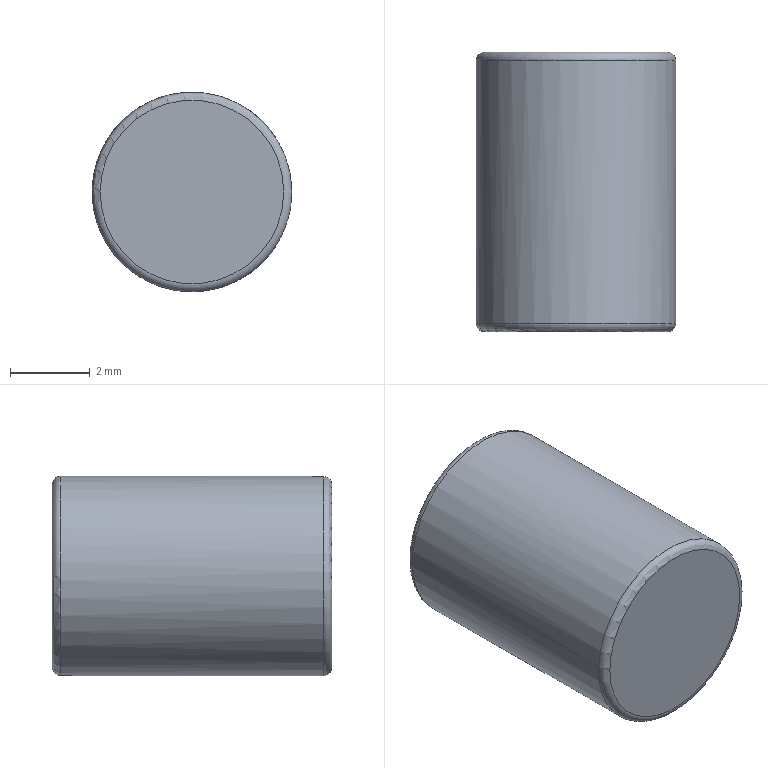Part | STEP file | Part [5] | 1 solid | 5 faces | box 5 x 7 x 5 mm | volume 137.18 mm3 | plane 2 | torus 2 | cylinder 1 | commonest cylinder face diameters 5 x1
STEP:
#1=CARTESIAN_POINT('',(-7.7,-134.3,0.));
#2=VERTEX_POINT('',#1);
#3=CARTESIAN_POINT('',(-10.,-134.3,0.));
#4=DIRECTION('',(0.,-1.,0.));
#5=DIRECTION('',(-1.,0.,0.));
#6=AXIS2_PLACEMENT_3D('',#3,#4,#5);
#7=CIRCLE('',#6,2.3);
#8=EDGE_CURVE('',#2,#2,#7,.T.);
#9=ORIENTED_EDGE('',*,*,#8,.T.);
#10=EDGE_LOOP('',(#9));
#11=FACE_BOUND('',#10,.T.);
#12=CARTESIAN_POINT('',(-10.,-134.3,0.));
#13=DIRECTION('',(0.,-1.,0.));
#14=DIRECTION('',(0.,0.,-1.));
#15=AXIS2_PLACEMENT_3D('',#12,#13,#14);
#16=PLANE('',#15);
#17=ADVANCED_FACE('',(#11),#16,.T.);
#18=CARTESIAN_POINT('',(-7.5,-134.1,0.));
#19=VERTEX_POINT('',#18);
#20=CARTESIAN_POINT('',(-7.5,-134.1,0.));
#21=CARTESIAN_POINT('',(-7.5,-134.1,0.05237));
#22=CARTESIAN_POINT('',(-7.503,-134.1,0.1571));
#23=CARTESIAN_POINT('',(-7.518,-134.1,0.3136));
#24=CARTESIAN_POINT('',(-7.543,-134.1,0.4688));
#25=CARTESIAN_POINT('',(-7.577,-134.1,0.6222));
#26=CARTESIAN_POINT('',(-7.621,-134.1,0.7732));
#27=CARTESIAN_POINT('',(-7.674,-134.1,0.9211));
#28=CARTESIAN_POINT('',(-7.737,-134.1,1.065));
#29=CARTESIAN_POINT('',(-7.808,-134.1,1.205));
#30=CARTESIAN_POINT('',(-7.888,-134.1,1.341));
#31=CARTESIAN_POINT('',(-7.976,-134.1,1.471));
#32=CARTESIAN_POINT('',(-8.073,-134.1,1.595));
#33=CARTESIAN_POINT('',(-8.177,-134.1,1.713));
#34=CARTESIAN_POINT('',(-8.288,-134.1,1.824));
#35=CARTESIAN_POINT('',(-8.406,-134.1,1.928));
#36=CARTESIAN_POINT('',(-8.53,-134.1,2.024));
#37=CARTESIAN_POINT('',(-8.66,-134.1,2.112));
#38=CARTESIAN_POINT('',(-8.795,-134.1,2.192));
#39=CARTESIAN_POINT('',(-8.935,-134.1,2.264));
#40=CARTESIAN_POINT('',(-9.08,-134.1,2.326));
#41=CARTESIAN_POINT('',(-9.227,-134.1,2.379));
#42=CARTESIAN_POINT('',(-9.378,-134.1,2.423));
#43=CARTESIAN_POINT('',(-9.532,-134.1,2.457));
#44=CARTESIAN_POINT('',(-9.687,-134.1,2.482));
#45=CARTESIAN_POINT('',(-9.844,-134.1,2.497));
#46=CARTESIAN_POINT('',(-10.001,-134.1,2.502));
#47=CARTESIAN_POINT('',(-10.158,-134.1,2.497));
#48=CARTESIAN_POINT('',(-10.314,-134.1,2.482));
#49=CARTESIAN_POINT('',(-10.469,-134.1,2.457));
#50=CARTESIAN_POINT('',(-10.623,-134.1,2.423));
#51=CARTESIAN_POINT('',(-10.774,-134.1,2.379));
#52=CARTESIAN_POINT('',(-10.922,-134.1,2.326));
#53=CARTESIAN_POINT('',(-11.066,-134.1,2.263));
#54=CARTESIAN_POINT('',(-11.206,-134.1,2.192));
#55=CARTESIAN_POINT('',(-11.341,-134.1,2.112));
#56=CARTESIAN_POINT('',(-11.471,-134.1,2.023));
#57=CARTESIAN_POINT('',(-11.595,-134.1,1.927));
#58=CARTESIAN_POINT('',(-11.713,-134.1,1.823));
#59=CARTESIAN_POINT('',(-11.824,-134.1,1.712));
#60=CARTESIAN_POINT('',(-11.928,-134.1,1.594));
#61=CARTESIAN_POINT('',(-12.024,-134.1,1.47));
#62=CARTESIAN_POINT('',(-12.113,-134.1,1.34));
#63=CARTESIAN_POINT('',(-12.193,-134.1,1.204));
#64=CARTESIAN_POINT('',(-12.264,-134.1,1.064));
#65=CARTESIAN_POINT('',(-12.326,-134.1,0.9199));
#66=CARTESIAN_POINT('',(-12.38,-134.1,0.772));
#67=CARTESIAN_POINT('',(-12.423,-134.1,0.621));
#68=CARTESIAN_POINT('',(-12.458,-134.1,0.4676));
#69=CARTESIAN_POINT('',(-12.482,-134.1,0.3123));
#70=CARTESIAN_POINT('',(-12.497,-134.1,0.1563));
#71=CARTESIAN_POINT('',(-12.5,-134.1,0.05195));
#72=CARTESIAN_POINT('',(-12.5,-134.1,0.));
#73=CARTESIAN_POINT('',(-12.5,-134.1,-0.05237));
#74=CARTESIAN_POINT('',(-12.497,-134.1,-0.1571));
#75=CARTESIAN_POINT('',(-12.482,-134.1,-0.3136));
#76=CARTESIAN_POINT('',(-12.457,-134.1,-0.4688));
#77=CARTESIAN_POINT('',(-12.423,-134.1,-0.6222));
#78=CARTESIAN_POINT('',(-12.379,-134.1,-0.7732));
#79=CARTESIAN_POINT('',(-12.326,-134.1,-0.9211));
#80=CARTESIAN_POINT('',(-12.263,-134.1,-1.065));
#81=CARTESIAN_POINT('',(-12.192,-134.1,-1.205));
#82=CARTESIAN_POINT('',(-12.112,-134.1,-1.341));
#83=CARTESIAN_POINT('',(-12.024,-134.1,-1.471));
#84=CARTESIAN_POINT('',(-11.927,-134.1,-1.595));
#85=CARTESIAN_POINT('',(-11.823,-134.1,-1.713));
#86=CARTESIAN_POINT('',(-11.712,-134.1,-1.824));
#87=CARTESIAN_POINT('',(-11.594,-134.1,-1.928));
#88=CARTESIAN_POINT('',(-11.47,-134.1,-2.024));
#89=CARTESIAN_POINT('',(-11.34,-134.1,-2.112));
#90=CARTESIAN_POINT('',(-11.205,-134.1,-2.192));
#91=CARTESIAN_POINT('',(-11.065,-134.1,-2.264));
#92=CARTESIAN_POINT('',(-10.92,-134.1,-2.326));
#93=CARTESIAN_POINT('',(-10.773,-134.1,-2.379));
#94=CARTESIAN_POINT('',(-10.622,-134.1,-2.423));
#95=CARTESIAN_POINT('',(-10.468,-134.1,-2.457));
#96=CARTESIAN_POINT('',(-10.313,-134.1,-2.482));
#97=CARTESIAN_POINT('',(-10.156,-134.1,-2.497));
#98=CARTESIAN_POINT('',(-9.999,-134.1,-2.502));
#99=CARTESIAN_POINT('',(-9.842,-134.1,-2.497));
#100=CARTESIAN_POINT('',(-9.686,-134.1,-2.482));
#101=CARTESIAN_POINT('',(-9.531,-134.1,-2.457));
#102=CARTESIAN_POINT('',(-9.377,-134.1,-2.423));
#103=CARTESIAN_POINT('',(-9.226,-134.1,-2.379));
#104=CARTESIAN_POINT('',(-9.078,-134.1,-2.326));
#105=CARTESIAN_POINT('',(-8.934,-134.1,-2.263));
#106=CARTESIAN_POINT('',(-8.794,-134.1,-2.192));
#107=CARTESIAN_POINT('',(-8.659,-134.1,-2.112));
#108=CARTESIAN_POINT('',(-8.529,-134.1,-2.023));
#109=CARTESIAN_POINT('',(-8.405,-134.1,-1.927));
#110=CARTESIAN_POINT('',(-8.287,-134.1,-1.823));
#111=CARTESIAN_POINT('',(-8.176,-134.1,-1.712));
#112=CARTESIAN_POINT('',(-8.072,-134.1,-1.594));
#113=CARTESIAN_POINT('',(-7.976,-134.1,-1.47));
#114=CARTESIAN_POINT('',(-7.887,-134.1,-1.34));
#115=CARTESIAN_POINT('',(-7.807,-134.1,-1.204));
#116=CARTESIAN_POINT('',(-7.736,-134.1,-1.064));
#117=CARTESIAN_POINT('',(-7.674,-134.1,-0.9199));
#118=CARTESIAN_POINT('',(-7.62,-134.1,-0.772));
#119=CARTESIAN_POINT('',(-7.577,-134.1,-0.621));
#120=CARTESIAN_POINT('',(-7.542,-134.1,-0.4676));
#121=CARTESIAN_POINT('',(-7.518,-134.1,-0.3123));
#122=CARTESIAN_POINT('',(-7.503,-134.1,-0.1563));
#123=CARTESIAN_POINT('',(-7.5,-134.1,-0.05195));
#124=CARTESIAN_POINT('',(-7.5,-134.1,0.));
#125=B_SPLINE_CURVE_WITH_KNOTS('',3,(#20,#21,#22,#23,#24,#25,#26,#27,#28,#29,#30,#31,#32,#33,#34,#35,#36,#37,#38,#39,#40,#41,#42,#43,#44,#45,#46,#47,#48,#49,#50,#51,#52,#53,#54,#55,#56,#57,#58,#59,#60,#61,#62,#63,#64,#65,#66,#67,#68,#69,#70,#71,#72,#73,#74,#75,#76,#77,#78,#79,#80,#81,#82,#83,#84,#85,#86,#87,#88,#89,#90,#91,#92,#93,#94,#95,#96,#97,#98,#99,#100,#101,#102,#103,#104,#105,#106,#107,#108,#109,#110,#111,#112,#113,#114,#115,#116,#117,#118,#119,#120,#121,#122,#123,#124),.UNSPECIFIED.,.T.,.F.,(4,1,1,1,1,1,1,1,1,1,1,1,1,1,1,1,1,1,1,1,1,1,1,1,1,1,1,1,1,1,1,1,1,1,1,1,1,1,1,1,1,1,1,1,1,1,1,1,1,1,3,1,1,1,1,1,1,1,1,1,1,1,1,1,1,1,1,1,1,1,1,1,1,1,1,1,1,1,1,1,1,1,1,1,1,1,1,1,1,1,1,1,1,1,1,1,1,1,1,1,4),(0.,0.01,0.02,0.03,0.04001,0.05001,0.06001,0.07001,0.08001,0.09001,0.1,0.11,0.12,0.13,0.14,0.15,0.16,0.17,0.18,0.19,0.2,0.21,0.22,0.23,0.24,0.25,0.26,0.27,0.28,0.29,0.3,0.31,0.3201,0.3301,0.3401,0.3501,0.3601,0.3701,0.3801,0.3901,0.4001,0.4101,0.4201,0.4301,0.4401,0.4501,0.4601,0.4701,0.4801,0.4901,0.5,0.51,0.52,0.53,0.54,0.55,0.56,0.57,0.58,0.59,0.6,0.61,0.62,0.63,0.64,0.65,0.66,0.67,0.68,0.69,0.7,0.71,0.72,0.73,0.74,0.75,0.76,0.77,0.78,0.79,0.8,0.81,0.8201,0.8301,0.8401,0.8501,0.8601,0.8701,0.8801,0.8901,0.9001,0.9101,0.9201,0.9301,0.9401,0.9501,0.9601,0.9701,0.9801,0.9901,1.),.UNSPECIFIED.);
#126=EDGE_CURVE('',#19,#19,#125,.T.);
#127=ORIENTED_EDGE('',*,*,#126,.T.);
#128=EDGE_LOOP('',(#127));
#129=FACE_OUTER_BOUND('',#128,.T.);
#130=ORIENTED_EDGE('',*,*,#8,.F.);
#131=EDGE_LOOP('',(#130));
#132=FACE_OUTER_BOUND('',#131,.T.);
#133=CARTESIAN_POINT('',(-10.,-134.1,0.));
#134=DIRECTION('',(0.,-1.,0.));
#135=DIRECTION('',(1.,0.,0.));
#136=AXIS2_PLACEMENT_3D('',#133,#134,#135);
#137=TOROIDAL_SURFACE('',#136,2.3,0.2);
#138=ADVANCED_FACE('',(#129,#132),#137,.T.);
#139=CARTESIAN_POINT('',(-7.5,-127.5,0.));
#140=VERTEX_POINT('',#139);
#141=CARTESIAN_POINT('',(-7.5,-127.5,0.));
#142=CARTESIAN_POINT('',(-7.5,-127.5,-0.05237));
#143=CARTESIAN_POINT('',(-7.503,-127.5,-0.1571));
#144=CARTESIAN_POINT('',(-7.518,-127.5,-0.3136));
#145=CARTESIAN_POINT('',(-7.543,-127.5,-0.4688));
#146=CARTESIAN_POINT('',(-7.577,-127.5,-0.6222));
#147=CARTESIAN_POINT('',(-7.621,-127.5,-0.7732));
#148=CARTESIAN_POINT('',(-7.674,-127.5,-0.9211));
#149=CARTESIAN_POINT('',(-7.737,-127.5,-1.065));
#150=CARTESIAN_POINT('',(-7.808,-127.5,-1.205));
#151=CARTESIAN_POINT('',(-7.888,-127.5,-1.341));
#152=CARTESIAN_POINT('',(-7.976,-127.5,-1.471));
#153=CARTESIAN_POINT('',(-8.073,-127.5,-1.595));
#154=CARTESIAN_POINT('',(-8.177,-127.5,-1.713));
#155=CARTESIAN_POINT('',(-8.288,-127.5,-1.824));
#156=CARTESIAN_POINT('',(-8.406,-127.5,-1.928));
#157=CARTESIAN_POINT('',(-8.53,-127.5,-2.024));
#158=CARTESIAN_POINT('',(-8.66,-127.5,-2.112));
#159=CARTESIAN_POINT('',(-8.795,-127.5,-2.192));
#160=CARTESIAN_POINT('',(-8.935,-127.5,-2.264));
#161=CARTESIAN_POINT('',(-9.08,-127.5,-2.326));
#162=CARTESIAN_POINT('',(-9.227,-127.5,-2.379));
#163=CARTESIAN_POINT('',(-9.378,-127.5,-2.423));
#164=CARTESIAN_POINT('',(-9.532,-127.5,-2.457));
#165=CARTESIAN_POINT('',(-9.687,-127.5,-2.482));
#166=CARTESIAN_POINT('',(-9.844,-127.5,-2.497));
#167=CARTESIAN_POINT('',(-10.001,-127.5,-2.502));
#168=CARTESIAN_POINT('',(-10.158,-127.5,-2.497));
#169=CARTESIAN_POINT('',(-10.314,-127.5,-2.482));
#170=CARTESIAN_POINT('',(-10.469,-127.5,-2.457));
#171=CARTESIAN_POINT('',(-10.623,-127.5,-2.423));
#172=CARTESIAN_POINT('',(-10.774,-127.5,-2.379));
#173=CARTESIAN_POINT('',(-10.922,-127.5,-2.326));
#174=CARTESIAN_POINT('',(-11.066,-127.5,-2.263));
#175=CARTESIAN_POINT('',(-11.206,-127.5,-2.192));
#176=CARTESIAN_POINT('',(-11.341,-127.5,-2.112));
#177=CARTESIAN_POINT('',(-11.471,-127.5,-2.023));
#178=CARTESIAN_POINT('',(-11.595,-127.5,-1.927));
#179=CARTESIAN_POINT('',(-11.713,-127.5,-1.823));
#180=CARTESIAN_POINT('',(-11.824,-127.5,-1.712));
#181=CARTESIAN_POINT('',(-11.928,-127.5,-1.594));
#182=CARTESIAN_POINT('',(-12.024,-127.5,-1.47));
#183=CARTESIAN_POINT('',(-12.113,-127.5,-1.34));
#184=CARTESIAN_POINT('',(-12.193,-127.5,-1.204));
#185=CARTESIAN_POINT('',(-12.264,-127.5,-1.064));
#186=CARTESIAN_POINT('',(-12.326,-127.5,-0.9199));
#187=CARTESIAN_POINT('',(-12.38,-127.5,-0.772));
#188=CARTESIAN_POINT('',(-12.423,-127.5,-0.621));
#189=CARTESIAN_POINT('',(-12.458,-127.5,-0.4676));
#190=CARTESIAN_POINT('',(-12.482,-127.5,-0.3123));
#191=CARTESIAN_POINT('',(-12.497,-127.5,-0.1563));
#192=CARTESIAN_POINT('',(-12.5,-127.5,-0.05195));
#193=CARTESIAN_POINT('',(-12.5,-127.5,0.));
#194=CARTESIAN_POINT('',(-12.5,-127.5,0.05237));
#195=CARTESIAN_POINT('',(-12.497,-127.5,0.1571));
#196=CARTESIAN_POINT('',(-12.482,-127.5,0.3136));
#197=CARTESIAN_POINT('',(-12.457,-127.5,0.4688));
#198=CARTESIAN_POINT('',(-12.423,-127.5,0.6222));
#199=CARTESIAN_POINT('',(-12.379,-127.5,0.7732));
#200=CARTESIAN_POINT('',(-12.326,-127.5,0.9211));
#201=CARTESIAN_POINT('',(-12.263,-127.5,1.065));
#202=CARTESIAN_POINT('',(-12.192,-127.5,1.205));
#203=CARTESIAN_POINT('',(-12.112,-127.5,1.341));
#204=CARTESIAN_POINT('',(-12.024,-127.5,1.471));
#205=CARTESIAN_POINT('',(-11.927,-127.5,1.595));
#206=CARTESIAN_POINT('',(-11.823,-127.5,1.713));
#207=CARTESIAN_POINT('',(-11.712,-127.5,1.824));
#208=CARTESIAN_POINT('',(-11.594,-127.5,1.928));
#209=CARTESIAN_POINT('',(-11.47,-127.5,2.024));
#210=CARTESIAN_POINT('',(-11.34,-127.5,2.112));
#211=CARTESIAN_POINT('',(-11.205,-127.5,2.192));
#212=CARTESIAN_POINT('',(-11.065,-127.5,2.264));
#213=CARTESIAN_POINT('',(-10.92,-127.5,2.326));
#214=CARTESIAN_POINT('',(-10.773,-127.5,2.379));
#215=CARTESIAN_POINT('',(-10.622,-127.5,2.423));
#216=CARTESIAN_POINT('',(-10.468,-127.5,2.457));
#217=CARTESIAN_POINT('',(-10.313,-127.5,2.482));
#218=CARTESIAN_POINT('',(-10.156,-127.5,2.497));
#219=CARTESIAN_POINT('',(-9.999,-127.5,2.502));
#220=CARTESIAN_POINT('',(-9.842,-127.5,2.497));
#221=CARTESIAN_POINT('',(-9.686,-127.5,2.482));
#222=CARTESIAN_POINT('',(-9.531,-127.5,2.457));
#223=CARTESIAN_POINT('',(-9.377,-127.5,2.423));
#224=CARTESIAN_POINT('',(-9.226,-127.5,2.379));
#225=CARTESIAN_POINT('',(-9.078,-127.5,2.326));
#226=CARTESIAN_POINT('',(-8.934,-127.5,2.263));
#227=CARTESIAN_POINT('',(-8.794,-127.5,2.192));
#228=CARTESIAN_POINT('',(-8.659,-127.5,2.112));
#229=CARTESIAN_POINT('',(-8.529,-127.5,2.023));
#230=CARTESIAN_POINT('',(-8.405,-127.5,1.927));
#231=CARTESIAN_POINT('',(-8.287,-127.5,1.823));
#232=CARTESIAN_POINT('',(-8.176,-127.5,1.712));
#233=CARTESIAN_POINT('',(-8.072,-127.5,1.594));
#234=CARTESIAN_POINT('',(-7.976,-127.5,1.47));
#235=CARTESIAN_POINT('',(-7.887,-127.5,1.34));
#236=CARTESIAN_POINT('',(-7.807,-127.5,1.204));
#237=CARTESIAN_POINT('',(-7.736,-127.5,1.064));
#238=CARTESIAN_POINT('',(-7.674,-127.5,0.9199));
#239=CARTESIAN_POINT('',(-7.62,-127.5,0.772));
#240=CARTESIAN_POINT('',(-7.577,-127.5,0.621));
#241=CARTESIAN_POINT('',(-7.542,-127.5,0.4676));
#242=CARTESIAN_POINT('',(-7.518,-127.5,0.3123));
#243=CARTESIAN_POINT('',(-7.503,-127.5,0.1563));
#244=CARTESIAN_POINT('',(-7.5,-127.5,0.05195));
#245=CARTESIAN_POINT('',(-7.5,-127.5,0.));
#246=B_SPLINE_CURVE_WITH_KNOTS('',3,(#141,#142,#143,#144,#145,#146,#147,#148,#149,#150,#151,#152,#153,#154,#155,#156,#157,#158,#159,#160,#161,#162,#163,#164,#165,#166,#167,#168,#169,#170,#171,#172,#173,#174,#175,#176,#177,#178,#179,#180,#181,#182,#183,#184,#185,#186,#187,#188,#189,#190,#191,#192,#193,#194,#195,#196,#197,#198,#199,#200,#201,#202,#203,#204,#205,#206,#207,#208,#209,#210,#211,#212,#213,#214,#215,#216,#217,#218,#219,#220,#221,#222,#223,#224,#225,#226,#227,#228,#229,#230,#231,#232,#233,#234,#235,#236,#237,#238,#239,#240,#241,#242,#243,#244,#245),.UNSPECIFIED.,.T.,.F.,(4,1,1,1,1,1,1,1,1,1,1,1,1,1,1,1,1,1,1,1,1,1,1,1,1,1,1,1,1,1,1,1,1,1,1,1,1,1,1,1,1,1,1,1,1,1,1,1,1,1,3,1,1,1,1,1,1,1,1,1,1,1,1,1,1,1,1,1,1,1,1,1,1,1,1,1,1,1,1,1,1,1,1,1,1,1,1,1,1,1,1,1,1,1,1,1,1,1,1,1,4),(0.,0.01,0.02,0.03,0.04001,0.05001,0.06001,0.07001,0.08001,0.09001,0.1,0.11,0.12,0.13,0.14,0.15,0.16,0.17,0.18,0.19,0.2,0.21,0.22,0.23,0.24,0.25,0.26,0.27,0.28,0.29,0.3,0.31,0.3201,0.3301,0.3401,0.3501,0.3601,0.3701,0.3801,0.3901,0.4001,0.4101,0.4201,0.4301,0.4401,0.4501,0.4601,0.4701,0.4801,0.4901,0.5,0.51,0.52,0.53,0.54,0.55,0.56,0.57,0.58,0.59,0.6,0.61,0.62,0.63,0.64,0.65,0.66,0.67,0.68,0.69,0.7,0.71,0.72,0.73,0.74,0.75,0.76,0.77,0.78,0.79,0.8,0.81,0.8201,0.8301,0.8401,0.8501,0.8601,0.8701,0.8801,0.8901,0.9001,0.9101,0.9201,0.9301,0.9401,0.9501,0.9601,0.9701,0.9801,0.9901,1.),.UNSPECIFIED.);
#247=EDGE_CURVE('',#140,#140,#246,.T.);
#248=ORIENTED_EDGE('',*,*,#247,.F.);
#249=EDGE_LOOP('',(#248));
#250=FACE_OUTER_BOUND('',#249,.T.);
#251=ORIENTED_EDGE('',*,*,#126,.F.);
#252=EDGE_LOOP('',(#251));
#253=FACE_OUTER_BOUND('',#252,.T.);
#254=CARTESIAN_POINT('',(-10.,-130.8,0.));
#255=DIRECTION('',(0.,-1.,0.));
#256=DIRECTION('',(1.,0.,0.));
#257=AXIS2_PLACEMENT_3D('',#254,#255,#256);
#258=CYLINDRICAL_SURFACE('',#257,2.5);
#259=ADVANCED_FACE('',(#250,#253),#258,.T.);
#260=ORIENTED_EDGE('',*,*,#247,.T.);
#261=EDGE_LOOP('',(#260));
#262=FACE_OUTER_BOUND('',#261,.T.);
#263=CARTESIAN_POINT('',(-7.7,-127.3,0.));
#264=VERTEX_POINT('',#263);
#265=CARTESIAN_POINT('',(-10.,-127.3,0.));
#266=DIRECTION('',(0.,-1.,0.));
#267=DIRECTION('',(-1.,0.,0.));
#268=AXIS2_PLACEMENT_3D('',#265,#266,#267);
#269=CIRCLE('',#268,2.3);
#270=EDGE_CURVE('',#264,#264,#269,.T.);
#271=ORIENTED_EDGE('',*,*,#270,.T.);
#272=EDGE_LOOP('',(#271));
#273=FACE_OUTER_BOUND('',#272,.T.);
#274=CARTESIAN_POINT('',(-10.,-127.5,0.));
#275=DIRECTION('',(0.,-1.,0.));
#276=DIRECTION('',(1.,0.,0.));
#277=AXIS2_PLACEMENT_3D('',#274,#275,#276);
#278=TOROIDAL_SURFACE('',#277,2.3,0.2);
#279=ADVANCED_FACE('',(#262,#273),#278,.T.);
#280=ORIENTED_EDGE('',*,*,#270,.F.);
#281=EDGE_LOOP('',(#280));
#282=FACE_BOUND('',#281,.T.);
#283=CARTESIAN_POINT('',(-10.,-127.3,0.));
#284=DIRECTION('',(0.,-1.,0.));
#285=DIRECTION('',(0.,0.,-1.));
#286=AXIS2_PLACEMENT_3D('',#283,#284,#285);
#287=PLANE('',#286);
#288=ADVANCED_FACE('',(#282),#287,.F.);
#289=CLOSED_SHELL('',(#17,#138,#259,#279,#288));
#290=MANIFOLD_SOLID_BREP('',#289);
#291=(LENGTH_UNIT()NAMED_UNIT(*)SI_UNIT(.MILLI.,.METRE.));
#292=UNCERTAINTY_MEASURE_WITH_UNIT(LENGTH_MEASURE(0.00001),#291,'','');
#293=(NAMED_UNIT(*)PLANE_ANGLE_UNIT()SI_UNIT($,.RADIAN.));
#294=(NAMED_UNIT(*)SI_UNIT($,.STERADIAN.)SOLID_ANGLE_UNIT());
#295=(GEOMETRIC_REPRESENTATION_CONTEXT(3)GLOBAL_UNCERTAINTY_ASSIGNED_CONTEXT((#292))GLOBAL_UNIT_ASSIGNED_CONTEXT((#291,#293,#294))REPRESENTATION_CONTEXT('',''));
#296=ADVANCED_BREP_SHAPE_REPRESENTATION('',(#290),#295);